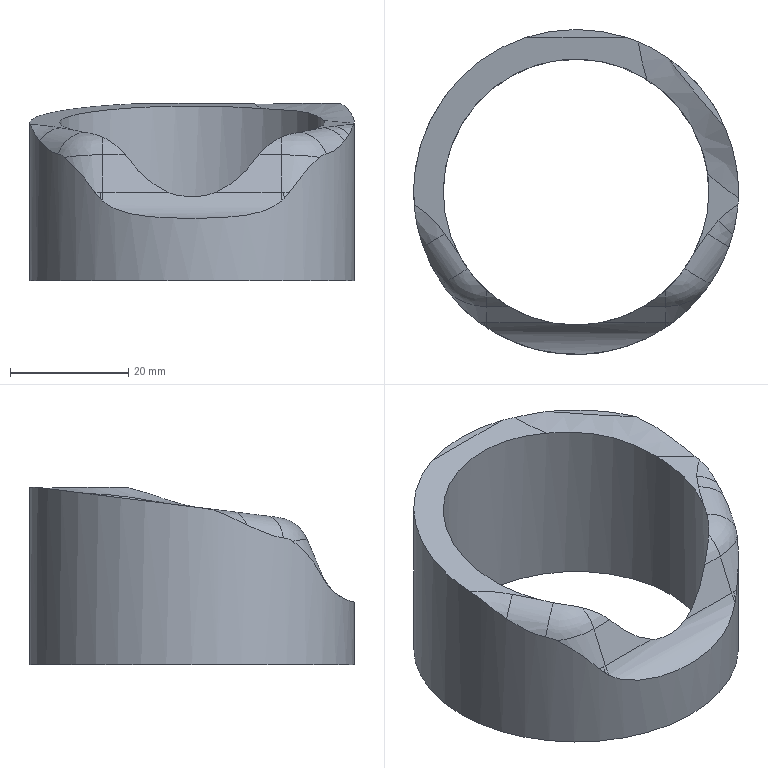Part | NX | features solid 2 | 1 solid | 26 faces | box 55 x 55 x 30 mm | volume 19238 mm3 | spline 10 | cylinder 9 | plane 7 | commonest cylinder face diameters 11.998 x2 12 x2 20 x2 15 x1 45 x1 55 x1